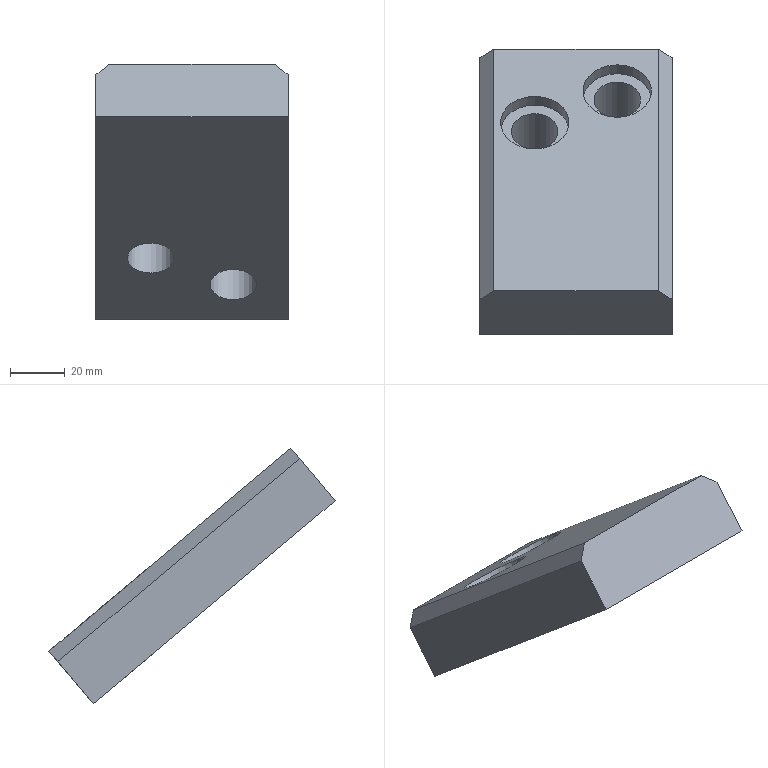Part | NX | features solid 2 | 1 solid | 14 faces | box 70 x 104.165 x 93.072 mm | volume 184387 mm3 | plane 10 | cylinder 4 | commonest cylinder face diameters 17 x2 25 x2
STEP:
#1=CARTESIAN_POINT('',(-265.,413.773,-31.941));
#2=VERTEX_POINT('',#1);
#3=CARTESIAN_POINT('',(-265.,400.917,-47.262));
#4=VERTEX_POINT('',#3);
#5=CARTESIAN_POINT('',(-265.,407.345,-39.602));
#6=DIRECTION('',(0.,-0.6428,-0.766));
#7=VECTOR('',#6,1000.);
#8=LINE('',#5,#7);
#9=EDGE_CURVE('',#2,#4,#8,.T.);
#10=ORIENTED_EDGE('',*,*,#9,.F.);
#11=CARTESIAN_POINT('',(-270.,416.987,-28.111));
#12=VERTEX_POINT('',#11);
#13=CARTESIAN_POINT('',(-280.,423.415,-20.45));
#14=DIRECTION('',(0.7071,-0.4545,-0.5417));
#15=VECTOR('',#14,1000.);
#16=LINE('',#13,#15);
#17=EDGE_CURVE('',#2,#12,#16,.F.);
#18=ORIENTED_EDGE('',*,*,#17,.T.);
#19=CARTESIAN_POINT('',(-330.,416.987,-28.111));
#20=VERTEX_POINT('',#19);
#21=CARTESIAN_POINT('',(-305.,416.987,-28.111));
#22=DIRECTION('',(1.,0.,0.));
#23=VECTOR('',#22,1000.);
#24=LINE('',#21,#23);
#25=EDGE_CURVE('',#20,#12,#24,.T.);
#26=ORIENTED_EDGE('',*,*,#25,.F.);
#27=CARTESIAN_POINT('',(-335.,413.773,-31.941));
#28=VERTEX_POINT('',#27);
#29=CARTESIAN_POINT('',(-325.,420.201,-24.281));
#30=DIRECTION('',(0.7071,0.4545,0.5417));
#31=VECTOR('',#30,1000.);
#32=LINE('',#29,#31);
#33=EDGE_CURVE('',#20,#28,#32,.F.);
#34=ORIENTED_EDGE('',*,*,#33,.T.);
#35=CARTESIAN_POINT('',(-335.,400.917,-47.262));
#36=VERTEX_POINT('',#35);
#37=CARTESIAN_POINT('',(-335.,407.345,-39.602));
#38=DIRECTION('',(0.,0.6428,0.766));
#39=VECTOR('',#38,1000.);
#40=LINE('',#37,#39);
#41=EDGE_CURVE('',#36,#28,#40,.T.);
#42=ORIENTED_EDGE('',*,*,#41,.F.);
#43=CARTESIAN_POINT('',(-305.,400.917,-47.262));
#44=DIRECTION('',(-1.,0.,0.));
#45=VECTOR('',#44,1000.);
#46=LINE('',#43,#45);
#47=EDGE_CURVE('',#4,#36,#46,.T.);
#48=ORIENTED_EDGE('',*,*,#47,.F.);
#49=EDGE_LOOP('',(#10,#18,#26,#34,#42,#48));
#50=FACE_BOUND('',#49,.T.);
#51=CARTESIAN_POINT('',(-305.,407.345,-39.602));
#52=DIRECTION('',(0.,-0.766,0.6428));
#53=DIRECTION('',(1.,0.,0.));
#54=AXIS2_PLACEMENT_3D('',#51,#52,#53);
#55=PLANE('',#54);
#56=ADVANCED_FACE('',(#50),#55,.T.);
#57=CARTESIAN_POINT('',(-315.,468.712,-104.149));
#58=VERTEX_POINT('',#57);
#59=CARTESIAN_POINT('',(-315.,462.201,-98.685));
#60=DIRECTION('',(0.,-0.6428,-0.766));
#61=DIRECTION('',(0.,0.766,-0.6428));
#62=AXIS2_PLACEMENT_3D('',#59,#60,#61);
#63=CIRCLE('',#62,8.5);
#64=EDGE_CURVE('',#58,#58,#63,.T.);
#65=ORIENTED_EDGE('',*,*,#64,.F.);
#66=EDGE_LOOP('',(#65));
#67=FACE_BOUND('',#66,.T.);
#68=CARTESIAN_POINT('',(-285.,480.203,-113.79));
#69=VERTEX_POINT('',#68);
#70=CARTESIAN_POINT('',(-285.,473.692,-108.327));
#71=DIRECTION('',(0.,-0.6428,-0.766));
#72=DIRECTION('',(0.,0.766,-0.6428));
#73=AXIS2_PLACEMENT_3D('',#70,#71,#72);
#74=CIRCLE('',#73,8.5);
#75=EDGE_CURVE('',#69,#69,#74,.T.);
#76=ORIENTED_EDGE('',*,*,#75,.F.);
#77=EDGE_LOOP('',(#76));
#78=FACE_BOUND('',#77,.T.);
#79=CARTESIAN_POINT('',(-265.,489.013,-121.183));
#80=VERTEX_POINT('',#79);
#81=CARTESIAN_POINT('',(-265.,420.069,-63.332));
#82=DIRECTION('',(0.,-0.766,0.6428));
#83=VECTOR('',#82,1000.);
#84=LINE('',#81,#83);
#85=EDGE_CURVE('',#80,#4,#84,.T.);
#86=ORIENTED_EDGE('',*,*,#85,.T.);
#87=ORIENTED_EDGE('',*,*,#47,.T.);
#88=CARTESIAN_POINT('',(-335.,489.013,-121.183));
#89=VERTEX_POINT('',#88);
#90=CARTESIAN_POINT('',(-335.,420.069,-63.332));
#91=DIRECTION('',(0.,-0.766,0.6428));
#92=VECTOR('',#91,1000.);
#93=LINE('',#90,#92);
#94=EDGE_CURVE('',#89,#36,#93,.T.);
#95=ORIENTED_EDGE('',*,*,#94,.F.);
#96=CARTESIAN_POINT('',(-305.,489.013,-121.183));
#97=DIRECTION('',(1.,0.,0.));
#98=VECTOR('',#97,1000.);
#99=LINE('',#96,#98);
#100=EDGE_CURVE('',#89,#80,#99,.T.);
#101=ORIENTED_EDGE('',*,*,#100,.T.);
#102=EDGE_LOOP('',(#86,#87,#95,#101));
#103=FACE_BOUND('',#102,.T.);
#104=CARTESIAN_POINT('',(-305.,420.069,-63.332));
#105=DIRECTION('',(0.,-0.6428,-0.766));
#106=DIRECTION('',(0.,0.766,-0.6428));
#107=AXIS2_PLACEMENT_3D('',#104,#105,#106);
#108=PLANE('',#107);
#109=ADVANCED_FACE('',(#67,#78,#103),#108,.T.);
#110=ORIENTED_EDGE('',*,*,#41,.T.);
#111=CARTESIAN_POINT('',(-335.,501.868,-105.862));
#112=VERTEX_POINT('',#111);
#113=CARTESIAN_POINT('',(-335.,432.924,-48.011));
#114=DIRECTION('',(0.,0.766,-0.6428));
#115=VECTOR('',#114,1000.);
#116=LINE('',#113,#115);
#117=EDGE_CURVE('',#28,#112,#116,.T.);
#118=ORIENTED_EDGE('',*,*,#117,.T.);
#119=CARTESIAN_POINT('',(-335.,495.44,-113.522));
#120=DIRECTION('',(0.,-0.6428,-0.766));
#121=VECTOR('',#120,1000.);
#122=LINE('',#119,#121);
#123=EDGE_CURVE('',#112,#89,#122,.T.);
#124=ORIENTED_EDGE('',*,*,#123,.T.);
#125=ORIENTED_EDGE('',*,*,#94,.T.);
#126=EDGE_LOOP('',(#110,#118,#124,#125));
#127=FACE_BOUND('',#126,.T.);
#128=CARTESIAN_POINT('',(-335.,426.496,-55.671));
#129=DIRECTION('',(-1.,0.,0.));
#130=DIRECTION('',(0.,-0.766,0.6428));
#131=AXIS2_PLACEMENT_3D('',#128,#129,#130);
#132=PLANE('',#131);
#133=ADVANCED_FACE('',(#127),#132,.T.);
#134=CARTESIAN_POINT('',(-315.,468.695,-71.499));
#135=VERTEX_POINT('',#134);
#136=CARTESIAN_POINT('',(-315.,478.271,-79.534));
#137=DIRECTION('',(0.,0.6428,0.766));
#138=DIRECTION('',(0.,-0.766,0.6428));
#139=AXIS2_PLACEMENT_3D('',#136,#137,#138);
#140=CIRCLE('',#139,12.5);
#141=EDGE_CURVE('',#135,#135,#140,.T.);
#142=ORIENTED_EDGE('',*,*,#141,.F.);
#143=EDGE_LOOP('',(#142));
#144=FACE_BOUND('',#143,.T.);
#145=CARTESIAN_POINT('',(-285.,480.186,-81.141));
#146=VERTEX_POINT('',#145);
#147=CARTESIAN_POINT('',(-285.,489.761,-89.176));
#148=DIRECTION('',(0.,0.6428,0.766));
#149=DIRECTION('',(0.,-0.766,0.6428));
#150=AXIS2_PLACEMENT_3D('',#147,#148,#149);
#151=CIRCLE('',#150,12.5);
#152=EDGE_CURVE('',#146,#146,#151,.T.);
#153=ORIENTED_EDGE('',*,*,#152,.F.);
#154=EDGE_LOOP('',(#153));
#155=FACE_BOUND('',#154,.T.);
#156=ORIENTED_EDGE('',*,*,#25,.T.);
#157=CARTESIAN_POINT('',(-270.,505.082,-102.031));
#158=VERTEX_POINT('',#157);
#159=CARTESIAN_POINT('',(-270.,436.138,-44.181));
#160=DIRECTION('',(0.,0.766,-0.6428));
#161=VECTOR('',#160,1000.);
#162=LINE('',#159,#161);
#163=EDGE_CURVE('',#12,#158,#162,.T.);
#164=ORIENTED_EDGE('',*,*,#163,.T.);
#165=CARTESIAN_POINT('',(-330.,505.082,-102.031));
#166=VERTEX_POINT('',#165);
#167=CARTESIAN_POINT('',(-305.,505.082,-102.031));
#168=DIRECTION('',(-1.,0.,0.));
#169=VECTOR('',#168,1000.);
#170=LINE('',#167,#169);
#171=EDGE_CURVE('',#158,#166,#170,.T.);
#172=ORIENTED_EDGE('',*,*,#171,.T.);
#173=CARTESIAN_POINT('',(-330.,436.138,-44.181));
#174=DIRECTION('',(0.,-0.766,0.6428));
#175=VECTOR('',#174,1000.);
#176=LINE('',#173,#175);
#177=EDGE_CURVE('',#166,#20,#176,.T.);
#178=ORIENTED_EDGE('',*,*,#177,.T.);
#179=EDGE_LOOP('',(#156,#164,#172,#178));
#180=FACE_BOUND('',#179,.T.);
#181=CARTESIAN_POINT('',(-305.,436.138,-44.181));
#182=DIRECTION('',(0.,0.6428,0.766));
#183=DIRECTION('',(0.,-0.766,0.6428));
#184=AXIS2_PLACEMENT_3D('',#181,#182,#183);
#185=PLANE('',#184);
#186=ADVANCED_FACE('',(#144,#155,#180),#185,.T.);
#187=ORIENTED_EDGE('',*,*,#171,.F.);
#188=CARTESIAN_POINT('',(-265.,501.868,-105.862));
#189=VERTEX_POINT('',#188);
#190=CARTESIAN_POINT('',(-280.,511.51,-94.371));
#191=DIRECTION('',(-0.7071,0.4545,0.5417));
#192=VECTOR('',#191,1000.);
#193=LINE('',#190,#192);
#194=EDGE_CURVE('',#158,#189,#193,.F.);
#195=ORIENTED_EDGE('',*,*,#194,.T.);
#196=CARTESIAN_POINT('',(-265.,495.44,-113.522));
#197=DIRECTION('',(0.,0.6428,0.766));
#198=VECTOR('',#197,1000.);
#199=LINE('',#196,#198);
#200=EDGE_CURVE('',#80,#189,#199,.T.);
#201=ORIENTED_EDGE('',*,*,#200,.F.);
#202=ORIENTED_EDGE('',*,*,#100,.F.);
#203=ORIENTED_EDGE('',*,*,#123,.F.);
#204=CARTESIAN_POINT('',(-325.,508.296,-98.201));
#205=DIRECTION('',(-0.7071,-0.4545,-0.5417));
#206=VECTOR('',#205,1000.);
#207=LINE('',#204,#206);
#208=EDGE_CURVE('',#112,#166,#207,.F.);
#209=ORIENTED_EDGE('',*,*,#208,.T.);
#210=EDGE_LOOP('',(#187,#195,#201,#202,#203,#209));
#211=FACE_BOUND('',#210,.T.);
#212=CARTESIAN_POINT('',(-305.,495.44,-113.522));
#213=DIRECTION('',(0.,0.766,-0.6428));
#214=DIRECTION('',(-1.,0.,0.));
#215=AXIS2_PLACEMENT_3D('',#212,#213,#214);
#216=PLANE('',#215);
#217=ADVANCED_FACE('',(#211),#216,.T.);
#218=ORIENTED_EDGE('',*,*,#200,.T.);
#219=CARTESIAN_POINT('',(-265.,432.924,-48.011));
#220=DIRECTION('',(0.,-0.766,0.6428));
#221=VECTOR('',#220,1000.);
#222=LINE('',#219,#221);
#223=EDGE_CURVE('',#189,#2,#222,.T.);
#224=ORIENTED_EDGE('',*,*,#223,.T.);
#225=ORIENTED_EDGE('',*,*,#9,.T.);
#226=ORIENTED_EDGE('',*,*,#85,.F.);
#227=EDGE_LOOP('',(#218,#224,#225,#226));
#228=FACE_BOUND('',#227,.T.);
#229=CARTESIAN_POINT('',(-265.,426.496,-55.671));
#230=DIRECTION('',(1.,0.,0.));
#231=DIRECTION('',(0.,0.766,-0.6428));
#232=AXIS2_PLACEMENT_3D('',#229,#230,#231);
#233=PLANE('',#232);
#234=ADVANCED_FACE('',(#228),#233,.T.);
#235=ORIENTED_EDGE('',*,*,#75,.T.);
#236=EDGE_LOOP('',(#235));
#237=FACE_BOUND('',#236,.T.);
#238=CARTESIAN_POINT('',(-285.,493.059,-98.47));
#239=VERTEX_POINT('',#238);
#240=CARTESIAN_POINT('',(-285.,486.547,-93.006));
#241=DIRECTION('',(0.,-0.6428,-0.766));
#242=DIRECTION('',(0.,0.766,-0.6428));
#243=AXIS2_PLACEMENT_3D('',#240,#241,#242);
#244=CIRCLE('',#243,8.5);
#245=EDGE_CURVE('',#239,#239,#244,.F.);
#246=ORIENTED_EDGE('',*,*,#245,.T.);
#247=EDGE_LOOP('',(#246));
#248=FACE_BOUND('',#247,.T.);
#249=CARTESIAN_POINT('',(-285.,464.05,-119.817));
#250=DIRECTION('',(0.,0.6428,0.766));
#251=DIRECTION('',(0.,-0.766,0.6428));
#252=AXIS2_PLACEMENT_3D('',#249,#250,#251);
#253=CYLINDRICAL_SURFACE('',#252,8.5);
#254=ADVANCED_FACE('',(#237,#248),#253,.F.);
#255=ORIENTED_EDGE('',*,*,#245,.F.);
#256=EDGE_LOOP('',(#255));
#257=FACE_BOUND('',#256,.T.);
#258=CARTESIAN_POINT('',(-285.,496.123,-101.041));
#259=VERTEX_POINT('',#258);
#260=CARTESIAN_POINT('',(-285.,486.547,-93.006));
#261=DIRECTION('',(0.,-0.6428,-0.766));
#262=DIRECTION('',(0.,0.766,-0.6428));
#263=AXIS2_PLACEMENT_3D('',#260,#261,#262);
#264=CIRCLE('',#263,12.5);
#265=EDGE_CURVE('',#259,#259,#264,.F.);
#266=ORIENTED_EDGE('',*,*,#265,.T.);
#267=EDGE_LOOP('',(#266));
#268=FACE_BOUND('',#267,.T.);
#269=CARTESIAN_POINT('',(-285.,486.547,-93.006));
#270=DIRECTION('',(0.,-0.6428,-0.766));
#271=DIRECTION('',(0.,0.766,-0.6428));
#272=AXIS2_PLACEMENT_3D('',#269,#270,#271);
#273=PLANE('',#272);
#274=ADVANCED_FACE('',(#257,#268),#273,.F.);
#275=ORIENTED_EDGE('',*,*,#152,.T.);
#276=EDGE_LOOP('',(#275));
#277=FACE_BOUND('',#276,.T.);
#278=ORIENTED_EDGE('',*,*,#265,.F.);
#279=EDGE_LOOP('',(#278));
#280=FACE_BOUND('',#279,.T.);
#281=CARTESIAN_POINT('',(-285.,483.333,-96.836));
#282=DIRECTION('',(0.,0.6428,0.766));
#283=DIRECTION('',(0.,-0.766,0.6428));
#284=AXIS2_PLACEMENT_3D('',#281,#282,#283);
#285=CYLINDRICAL_SURFACE('',#284,12.5);
#286=ADVANCED_FACE('',(#277,#280),#285,.F.);
#287=ORIENTED_EDGE('',*,*,#64,.T.);
#288=EDGE_LOOP('',(#287));
#289=FACE_BOUND('',#288,.T.);
#290=CARTESIAN_POINT('',(-315.,481.568,-88.828));
#291=VERTEX_POINT('',#290);
#292=CARTESIAN_POINT('',(-315.,475.057,-83.364));
#293=DIRECTION('',(0.,-0.6428,-0.766));
#294=DIRECTION('',(0.,0.766,-0.6428));
#295=AXIS2_PLACEMENT_3D('',#292,#293,#294);
#296=CIRCLE('',#295,8.5);
#297=EDGE_CURVE('',#291,#291,#296,.F.);
#298=ORIENTED_EDGE('',*,*,#297,.T.);
#299=EDGE_LOOP('',(#298));
#300=FACE_BOUND('',#299,.T.);
#301=CARTESIAN_POINT('',(-315.,452.559,-110.176));
#302=DIRECTION('',(0.,0.6428,0.766));
#303=DIRECTION('',(0.,-0.766,0.6428));
#304=AXIS2_PLACEMENT_3D('',#301,#302,#303);
#305=CYLINDRICAL_SURFACE('',#304,8.5);
#306=ADVANCED_FACE('',(#289,#300),#305,.F.);
#307=ORIENTED_EDGE('',*,*,#297,.F.);
#308=EDGE_LOOP('',(#307));
#309=FACE_BOUND('',#308,.T.);
#310=CARTESIAN_POINT('',(-315.,484.632,-91.399));
#311=VERTEX_POINT('',#310);
#312=CARTESIAN_POINT('',(-315.,475.057,-83.364));
#313=DIRECTION('',(0.,-0.6428,-0.766));
#314=DIRECTION('',(0.,0.766,-0.6428));
#315=AXIS2_PLACEMENT_3D('',#312,#313,#314);
#316=CIRCLE('',#315,12.5);
#317=EDGE_CURVE('',#311,#311,#316,.F.);
#318=ORIENTED_EDGE('',*,*,#317,.T.);
#319=EDGE_LOOP('',(#318));
#320=FACE_BOUND('',#319,.T.);
#321=CARTESIAN_POINT('',(-315.,475.057,-83.364));
#322=DIRECTION('',(0.,-0.6428,-0.766));
#323=DIRECTION('',(0.,0.766,-0.6428));
#324=AXIS2_PLACEMENT_3D('',#321,#322,#323);
#325=PLANE('',#324);
#326=ADVANCED_FACE('',(#309,#320),#325,.F.);
#327=ORIENTED_EDGE('',*,*,#141,.T.);
#328=EDGE_LOOP('',(#327));
#329=FACE_BOUND('',#328,.T.);
#330=ORIENTED_EDGE('',*,*,#317,.F.);
#331=EDGE_LOOP('',(#330));
#332=FACE_BOUND('',#331,.T.);
#333=CARTESIAN_POINT('',(-315.,471.843,-87.194));
#334=DIRECTION('',(0.,0.6428,0.766));
#335=DIRECTION('',(0.,-0.766,0.6428));
#336=AXIS2_PLACEMENT_3D('',#333,#334,#335);
#337=CYLINDRICAL_SURFACE('',#336,12.5);
#338=ADVANCED_FACE('',(#329,#332),#337,.F.);
#339=ORIENTED_EDGE('',*,*,#194,.F.);
#340=ORIENTED_EDGE('',*,*,#163,.F.);
#341=ORIENTED_EDGE('',*,*,#17,.F.);
#342=ORIENTED_EDGE('',*,*,#223,.F.);
#343=EDGE_LOOP('',(#339,#340,#341,#342));
#344=FACE_BOUND('',#343,.T.);
#345=CARTESIAN_POINT('',(-265.,432.924,-48.011));
#346=DIRECTION('',(-0.7071,-0.4545,-0.5417));
#347=DIRECTION('',(-0.6081,0.,0.7938));
#348=AXIS2_PLACEMENT_3D('',#345,#346,#347);
#349=PLANE('',#348);
#350=ADVANCED_FACE('',(#344),#349,.F.);
#351=ORIENTED_EDGE('',*,*,#208,.F.);
#352=ORIENTED_EDGE('',*,*,#117,.F.);
#353=ORIENTED_EDGE('',*,*,#33,.F.);
#354=ORIENTED_EDGE('',*,*,#177,.F.);
#355=EDGE_LOOP('',(#351,#352,#353,#354));
#356=FACE_BOUND('',#355,.T.);
#357=CARTESIAN_POINT('',(-330.,436.138,-44.181));
#358=DIRECTION('',(0.7071,-0.4545,-0.5417));
#359=DIRECTION('',(-0.6081,0.,-0.7938));
#360=AXIS2_PLACEMENT_3D('',#357,#358,#359);
#361=PLANE('',#360);
#362=ADVANCED_FACE('',(#356),#361,.F.);
#363=CLOSED_SHELL('',(#56,#109,#133,#186,#217,#234,#254,#274,#286,#306,#326,#338,#350,#362));
#364=MANIFOLD_SOLID_BREP('',#363);
#365=(LENGTH_UNIT()NAMED_UNIT(*)SI_UNIT(.MILLI.,.METRE.));
#366=UNCERTAINTY_MEASURE_WITH_UNIT(LENGTH_MEASURE(0.00001),#365,'','');
#367=(NAMED_UNIT(*)PLANE_ANGLE_UNIT()SI_UNIT($,.RADIAN.));
#368=(NAMED_UNIT(*)SI_UNIT($,.STERADIAN.)SOLID_ANGLE_UNIT());
#369=(GEOMETRIC_REPRESENTATION_CONTEXT(3)GLOBAL_UNCERTAINTY_ASSIGNED_CONTEXT((#366))GLOBAL_UNIT_ASSIGNED_CONTEXT((#365,#367,#368))REPRESENTATION_CONTEXT('',''));
#370=ADVANCED_BREP_SHAPE_REPRESENTATION('',(#364),#369);